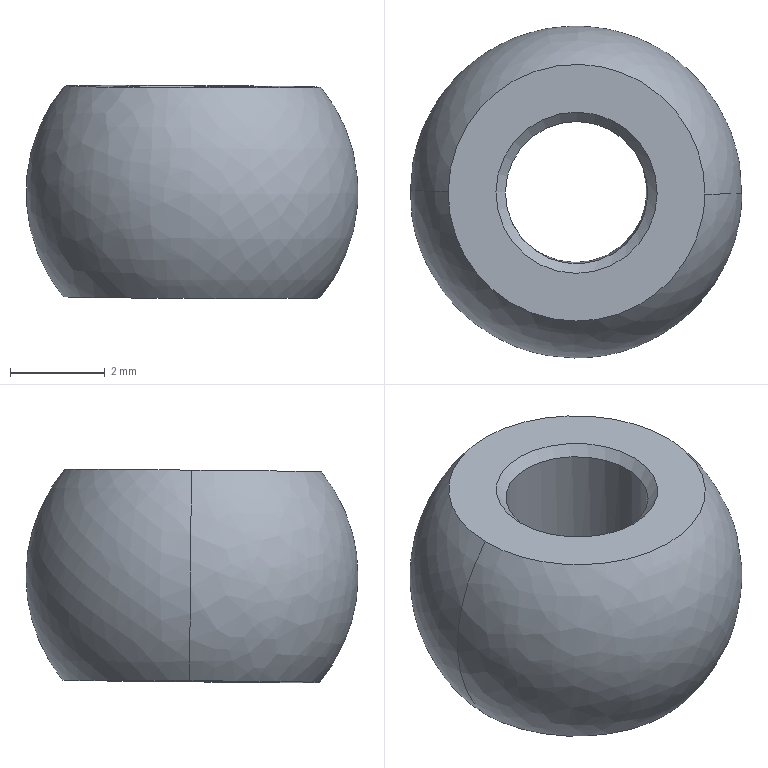Part | STEP file | Spare ball joint-1 | 1 solid | 7 faces | box 7 x 7 x 4.494 mm | volume 116.194 mm3 | spline 2 | cone 2 | plane 2 | cylinder 1 | commonest cylinder face diameters 3 x1